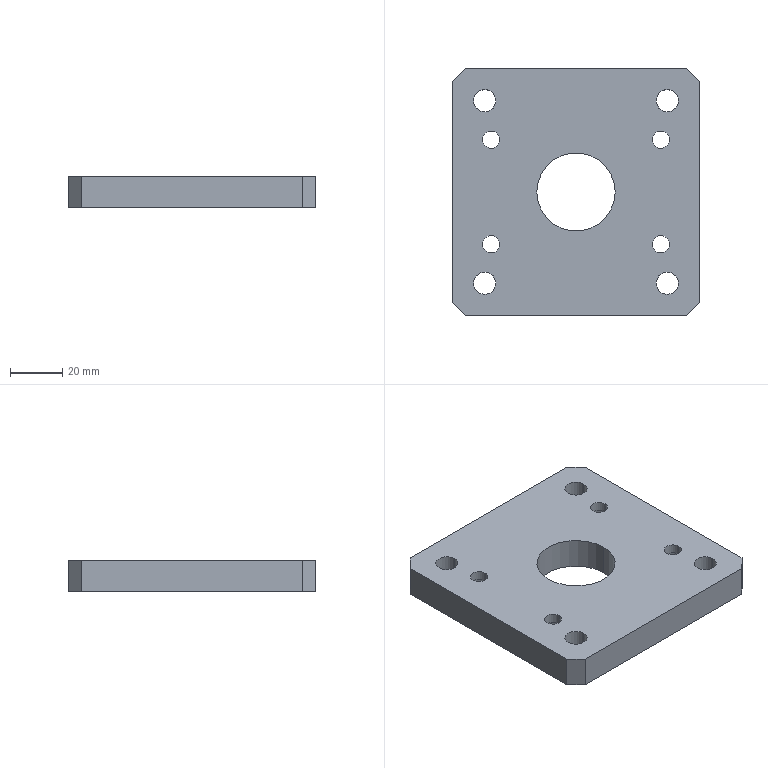Part | SolidWorks | features 3DProfileFeature 3, HoleWzd 3, Chamfer 1, Extrusion 1, ICE 1 | 1 solid | 40 faces | box 95 x 95 x 12 mm | volume 92833 mm3 | cylinder 26 | plane 14 | commonest cylinder face diameters 6.6 x8 8.5 x8 11 x8 30 x2
STEP:
#1=CARTESIAN_POINT('',(87.554,35.,12.));
#2=VERTEX_POINT('',#1);
#3=CARTESIAN_POINT('',(79.054,35.,12.));
#4=VERTEX_POINT('',#3);
#5=CARTESIAN_POINT('',(83.304,35.,12.));
#6=DIRECTION('',(0.,0.,-1.));
#7=DIRECTION('',(-1.,0.,0.));
#8=AXIS2_PLACEMENT_3D('',#5,#6,#7);
#9=CIRCLE('',#8,4.25);
#10=EDGE_CURVE('',#2,#4,#9,.T.);
#11=ORIENTED_EDGE('',*,*,#10,.F.);
#12=CARTESIAN_POINT('',(87.554,35.,0.));
#13=VERTEX_POINT('',#12);
#14=CARTESIAN_POINT('',(87.554,35.,0.));
#15=DIRECTION('',(0.,0.,-1.));
#16=VECTOR('',#15,1000.);
#17=LINE('',#14,#16);
#18=EDGE_CURVE('',#2,#13,#17,.T.);
#19=ORIENTED_EDGE('',*,*,#18,.T.);
#20=CARTESIAN_POINT('',(79.054,35.,0.));
#21=VERTEX_POINT('',#20);
#22=CARTESIAN_POINT('',(83.304,35.,0.));
#23=DIRECTION('',(0.,0.,-1.));
#24=DIRECTION('',(-1.,0.,0.));
#25=AXIS2_PLACEMENT_3D('',#22,#23,#24);
#26=CIRCLE('',#25,4.25);
#27=EDGE_CURVE('',#13,#21,#26,.T.);
#28=ORIENTED_EDGE('',*,*,#27,.T.);
#29=CARTESIAN_POINT('',(79.054,35.,0.));
#30=DIRECTION('',(0.,0.,-1.));
#31=VECTOR('',#30,1000.);
#32=LINE('',#29,#31);
#33=EDGE_CURVE('',#4,#21,#32,.T.);
#34=ORIENTED_EDGE('',*,*,#33,.F.);
#35=EDGE_LOOP('',(#11,#19,#28,#34));
#36=FACE_OUTER_BOUND('',#35,.T.);
#37=CARTESIAN_POINT('',(83.304,35.,0.));
#38=DIRECTION('',(0.,0.,-1.));
#39=DIRECTION('',(-1.,0.,0.));
#40=AXIS2_PLACEMENT_3D('',#37,#38,#39);
#41=CYLINDRICAL_SURFACE('',#40,4.25);
#42=ADVANCED_FACE('',(#36),#41,.F.);
#43=CARTESIAN_POINT('',(17.554,35.,12.));
#44=VERTEX_POINT('',#43);
#45=CARTESIAN_POINT('',(9.054,35.,12.));
#46=VERTEX_POINT('',#45);
#47=CARTESIAN_POINT('',(13.304,35.,12.));
#48=DIRECTION('',(0.,0.,-1.));
#49=DIRECTION('',(-1.,0.,0.));
#50=AXIS2_PLACEMENT_3D('',#47,#48,#49);
#51=CIRCLE('',#50,4.25);
#52=EDGE_CURVE('',#44,#46,#51,.T.);
#53=ORIENTED_EDGE('',*,*,#52,.F.);
#54=CARTESIAN_POINT('',(17.554,35.,0.));
#55=VERTEX_POINT('',#54);
#56=CARTESIAN_POINT('',(17.554,35.,0.));
#57=DIRECTION('',(0.,0.,-1.));
#58=VECTOR('',#57,1000.);
#59=LINE('',#56,#58);
#60=EDGE_CURVE('',#44,#55,#59,.T.);
#61=ORIENTED_EDGE('',*,*,#60,.T.);
#62=CARTESIAN_POINT('',(9.054,35.,0.));
#63=VERTEX_POINT('',#62);
#64=CARTESIAN_POINT('',(13.304,35.,0.));
#65=DIRECTION('',(0.,0.,-1.));
#66=DIRECTION('',(-1.,0.,0.));
#67=AXIS2_PLACEMENT_3D('',#64,#65,#66);
#68=CIRCLE('',#67,4.25);
#69=EDGE_CURVE('',#55,#63,#68,.T.);
#70=ORIENTED_EDGE('',*,*,#69,.T.);
#71=CARTESIAN_POINT('',(9.054,35.,0.));
#72=DIRECTION('',(0.,0.,-1.));
#73=VECTOR('',#72,1000.);
#74=LINE('',#71,#73);
#75=EDGE_CURVE('',#46,#63,#74,.T.);
#76=ORIENTED_EDGE('',*,*,#75,.F.);
#77=EDGE_LOOP('',(#53,#61,#70,#76));
#78=FACE_OUTER_BOUND('',#77,.T.);
#79=CARTESIAN_POINT('',(13.304,35.,0.));
#80=DIRECTION('',(0.,0.,-1.));
#81=DIRECTION('',(-1.,0.,0.));
#82=AXIS2_PLACEMENT_3D('',#79,#80,#81);
#83=CYLINDRICAL_SURFACE('',#82,4.25);
#84=ADVANCED_FACE('',(#78),#83,.F.);
#85=CARTESIAN_POINT('',(17.554,-35.,12.));
#86=VERTEX_POINT('',#85);
#87=CARTESIAN_POINT('',(9.054,-35.,12.));
#88=VERTEX_POINT('',#87);
#89=CARTESIAN_POINT('',(13.304,-35.,12.));
#90=DIRECTION('',(0.,0.,-1.));
#91=DIRECTION('',(-1.,0.,0.));
#92=AXIS2_PLACEMENT_3D('',#89,#90,#91);
#93=CIRCLE('',#92,4.25);
#94=EDGE_CURVE('',#86,#88,#93,.T.);
#95=ORIENTED_EDGE('',*,*,#94,.F.);
#96=CARTESIAN_POINT('',(17.554,-35.,0.));
#97=VERTEX_POINT('',#96);
#98=CARTESIAN_POINT('',(17.554,-35.,0.));
#99=DIRECTION('',(0.,0.,-1.));
#100=VECTOR('',#99,1000.);
#101=LINE('',#98,#100);
#102=EDGE_CURVE('',#86,#97,#101,.T.);
#103=ORIENTED_EDGE('',*,*,#102,.T.);
#104=CARTESIAN_POINT('',(9.054,-35.,0.));
#105=VERTEX_POINT('',#104);
#106=CARTESIAN_POINT('',(13.304,-35.,0.));
#107=DIRECTION('',(0.,0.,-1.));
#108=DIRECTION('',(-1.,0.,0.));
#109=AXIS2_PLACEMENT_3D('',#106,#107,#108);
#110=CIRCLE('',#109,4.25);
#111=EDGE_CURVE('',#97,#105,#110,.T.);
#112=ORIENTED_EDGE('',*,*,#111,.T.);
#113=CARTESIAN_POINT('',(9.054,-35.,0.));
#114=DIRECTION('',(0.,0.,-1.));
#115=VECTOR('',#114,1000.);
#116=LINE('',#113,#115);
#117=EDGE_CURVE('',#88,#105,#116,.T.);
#118=ORIENTED_EDGE('',*,*,#117,.F.);
#119=EDGE_LOOP('',(#95,#103,#112,#118));
#120=FACE_OUTER_BOUND('',#119,.T.);
#121=CARTESIAN_POINT('',(13.304,-35.,0.));
#122=DIRECTION('',(0.,0.,-1.));
#123=DIRECTION('',(-1.,0.,0.));
#124=AXIS2_PLACEMENT_3D('',#121,#122,#123);
#125=CYLINDRICAL_SURFACE('',#124,4.25);
#126=ADVANCED_FACE('',(#120),#125,.F.);
#127=CARTESIAN_POINT('',(87.554,-35.,12.));
#128=VERTEX_POINT('',#127);
#129=CARTESIAN_POINT('',(79.054,-35.,12.));
#130=VERTEX_POINT('',#129);
#131=CARTESIAN_POINT('',(83.304,-35.,12.));
#132=DIRECTION('',(0.,0.,-1.));
#133=DIRECTION('',(-1.,0.,0.));
#134=AXIS2_PLACEMENT_3D('',#131,#132,#133);
#135=CIRCLE('',#134,4.25);
#136=EDGE_CURVE('',#128,#130,#135,.T.);
#137=ORIENTED_EDGE('',*,*,#136,.F.);
#138=CARTESIAN_POINT('',(87.554,-35.,0.));
#139=VERTEX_POINT('',#138);
#140=CARTESIAN_POINT('',(87.554,-35.,0.));
#141=DIRECTION('',(0.,0.,-1.));
#142=VECTOR('',#141,1000.);
#143=LINE('',#140,#142);
#144=EDGE_CURVE('',#128,#139,#143,.T.);
#145=ORIENTED_EDGE('',*,*,#144,.T.);
#146=CARTESIAN_POINT('',(79.054,-35.,0.));
#147=VERTEX_POINT('',#146);
#148=CARTESIAN_POINT('',(83.304,-35.,0.));
#149=DIRECTION('',(0.,0.,-1.));
#150=DIRECTION('',(-1.,0.,0.));
#151=AXIS2_PLACEMENT_3D('',#148,#149,#150);
#152=CIRCLE('',#151,4.25);
#153=EDGE_CURVE('',#139,#147,#152,.T.);
#154=ORIENTED_EDGE('',*,*,#153,.T.);
#155=CARTESIAN_POINT('',(79.054,-35.,0.));
#156=DIRECTION('',(0.,0.,-1.));
#157=VECTOR('',#156,1000.);
#158=LINE('',#155,#157);
#159=EDGE_CURVE('',#130,#147,#158,.T.);
#160=ORIENTED_EDGE('',*,*,#159,.F.);
#161=EDGE_LOOP('',(#137,#145,#154,#160));
#162=FACE_OUTER_BOUND('',#161,.T.);
#163=CARTESIAN_POINT('',(83.304,-35.,0.));
#164=DIRECTION('',(0.,0.,-1.));
#165=DIRECTION('',(-1.,0.,0.));
#166=AXIS2_PLACEMENT_3D('',#163,#164,#165);
#167=CYLINDRICAL_SURFACE('',#166,4.25);
#168=ADVANCED_FACE('',(#162),#167,.F.);
#169=CARTESIAN_POINT('',(86.304,20.,8.3));
#170=VERTEX_POINT('',#169);
#171=CARTESIAN_POINT('',(75.304,20.,8.3));
#172=VERTEX_POINT('',#171);
#173=CARTESIAN_POINT('',(80.804,20.,8.3));
#174=DIRECTION('',(0.,0.,-1.));
#175=DIRECTION('',(-1.,0.,0.));
#176=AXIS2_PLACEMENT_3D('',#173,#174,#175);
#177=CIRCLE('',#176,5.5);
#178=EDGE_CURVE('',#170,#172,#177,.T.);
#179=ORIENTED_EDGE('',*,*,#178,.F.);
#180=CARTESIAN_POINT('',(86.304,20.,0.));
#181=VERTEX_POINT('',#180);
#182=CARTESIAN_POINT('',(86.304,20.,0.));
#183=DIRECTION('',(0.,0.,-1.));
#184=VECTOR('',#183,1000.);
#185=LINE('',#182,#184);
#186=EDGE_CURVE('',#170,#181,#185,.T.);
#187=ORIENTED_EDGE('',*,*,#186,.T.);
#188=CARTESIAN_POINT('',(75.304,20.,0.));
#189=VERTEX_POINT('',#188);
#190=CARTESIAN_POINT('',(80.804,20.,0.));
#191=DIRECTION('',(0.,0.,-1.));
#192=DIRECTION('',(-1.,0.,0.));
#193=AXIS2_PLACEMENT_3D('',#190,#191,#192);
#194=CIRCLE('',#193,5.5);
#195=EDGE_CURVE('',#181,#189,#194,.T.);
#196=ORIENTED_EDGE('',*,*,#195,.T.);
#197=CARTESIAN_POINT('',(75.304,20.,0.));
#198=DIRECTION('',(0.,0.,-1.));
#199=VECTOR('',#198,1000.);
#200=LINE('',#197,#199);
#201=EDGE_CURVE('',#172,#189,#200,.T.);
#202=ORIENTED_EDGE('',*,*,#201,.F.);
#203=EDGE_LOOP('',(#179,#187,#196,#202));
#204=FACE_OUTER_BOUND('',#203,.T.);
#205=CARTESIAN_POINT('',(80.804,20.,0.));
#206=DIRECTION('',(0.,0.,-1.));
#207=DIRECTION('',(-1.,0.,0.));
#208=AXIS2_PLACEMENT_3D('',#205,#206,#207);
#209=CYLINDRICAL_SURFACE('',#208,5.5);
#210=ADVANCED_FACE('',(#204),#209,.F.);
#211=CARTESIAN_POINT('',(84.104,20.,12.));
#212=VERTEX_POINT('',#211);
#213=CARTESIAN_POINT('',(77.504,20.,12.));
#214=VERTEX_POINT('',#213);
#215=CARTESIAN_POINT('',(80.804,20.,12.));
#216=DIRECTION('',(0.,0.,-1.));
#217=DIRECTION('',(-1.,0.,0.));
#218=AXIS2_PLACEMENT_3D('',#215,#216,#217);
#219=CIRCLE('',#218,3.3);
#220=EDGE_CURVE('',#212,#214,#219,.T.);
#221=ORIENTED_EDGE('',*,*,#220,.F.);
#222=CARTESIAN_POINT('',(84.104,20.,8.3));
#223=VERTEX_POINT('',#222);
#224=CARTESIAN_POINT('',(84.104,20.,0.));
#225=DIRECTION('',(0.,0.,-1.));
#226=VECTOR('',#225,1000.);
#227=LINE('',#224,#226);
#228=EDGE_CURVE('',#212,#223,#227,.T.);
#229=ORIENTED_EDGE('',*,*,#228,.T.);
#230=CARTESIAN_POINT('',(77.504,20.,8.3));
#231=VERTEX_POINT('',#230);
#232=CARTESIAN_POINT('',(80.804,20.,8.3));
#233=DIRECTION('',(0.,0.,-1.));
#234=DIRECTION('',(-1.,0.,0.));
#235=AXIS2_PLACEMENT_3D('',#232,#233,#234);
#236=CIRCLE('',#235,3.3);
#237=EDGE_CURVE('',#223,#231,#236,.T.);
#238=ORIENTED_EDGE('',*,*,#237,.T.);
#239=CARTESIAN_POINT('',(77.504,20.,0.));
#240=DIRECTION('',(0.,0.,-1.));
#241=VECTOR('',#240,1000.);
#242=LINE('',#239,#241);
#243=EDGE_CURVE('',#214,#231,#242,.T.);
#244=ORIENTED_EDGE('',*,*,#243,.F.);
#245=EDGE_LOOP('',(#221,#229,#238,#244));
#246=FACE_OUTER_BOUND('',#245,.T.);
#247=CARTESIAN_POINT('',(80.804,20.,0.));
#248=DIRECTION('',(0.,0.,-1.));
#249=DIRECTION('',(-1.,0.,0.));
#250=AXIS2_PLACEMENT_3D('',#247,#248,#249);
#251=CYLINDRICAL_SURFACE('',#250,3.3);
#252=ADVANCED_FACE('',(#246),#251,.F.);
#253=CARTESIAN_POINT('',(21.304,20.,8.3));
#254=VERTEX_POINT('',#253);
#255=CARTESIAN_POINT('',(10.304,20.,8.3));
#256=VERTEX_POINT('',#255);
#257=CARTESIAN_POINT('',(15.804,20.,8.3));
#258=DIRECTION('',(0.,0.,-1.));
#259=DIRECTION('',(-1.,0.,0.));
#260=AXIS2_PLACEMENT_3D('',#257,#258,#259);
#261=CIRCLE('',#260,5.5);
#262=EDGE_CURVE('',#254,#256,#261,.T.);
#263=ORIENTED_EDGE('',*,*,#262,.F.);
#264=CARTESIAN_POINT('',(21.304,20.,0.));
#265=VERTEX_POINT('',#264);
#266=CARTESIAN_POINT('',(21.304,20.,0.));
#267=DIRECTION('',(0.,0.,-1.));
#268=VECTOR('',#267,1000.);
#269=LINE('',#266,#268);
#270=EDGE_CURVE('',#254,#265,#269,.T.);
#271=ORIENTED_EDGE('',*,*,#270,.T.);
#272=CARTESIAN_POINT('',(10.304,20.,0.));
#273=VERTEX_POINT('',#272);
#274=CARTESIAN_POINT('',(15.804,20.,0.));
#275=DIRECTION('',(0.,0.,-1.));
#276=DIRECTION('',(-1.,0.,0.));
#277=AXIS2_PLACEMENT_3D('',#274,#275,#276);
#278=CIRCLE('',#277,5.5);
#279=EDGE_CURVE('',#265,#273,#278,.T.);
#280=ORIENTED_EDGE('',*,*,#279,.T.);
#281=CARTESIAN_POINT('',(10.304,20.,0.));
#282=DIRECTION('',(0.,0.,-1.));
#283=VECTOR('',#282,1000.);
#284=LINE('',#281,#283);
#285=EDGE_CURVE('',#256,#273,#284,.T.);
#286=ORIENTED_EDGE('',*,*,#285,.F.);
#287=EDGE_LOOP('',(#263,#271,#280,#286));
#288=FACE_OUTER_BOUND('',#287,.T.);
#289=CARTESIAN_POINT('',(15.804,20.,0.));
#290=DIRECTION('',(0.,0.,-1.));
#291=DIRECTION('',(-1.,0.,0.));
#292=AXIS2_PLACEMENT_3D('',#289,#290,#291);
#293=CYLINDRICAL_SURFACE('',#292,5.5);
#294=ADVANCED_FACE('',(#288),#293,.F.);
#295=CARTESIAN_POINT('',(19.104,20.,12.));
#296=VERTEX_POINT('',#295);
#297=CARTESIAN_POINT('',(12.504,20.,12.));
#298=VERTEX_POINT('',#297);
#299=CARTESIAN_POINT('',(15.804,20.,12.));
#300=DIRECTION('',(0.,0.,-1.));
#301=DIRECTION('',(-1.,0.,0.));
#302=AXIS2_PLACEMENT_3D('',#299,#300,#301);
#303=CIRCLE('',#302,3.3);
#304=EDGE_CURVE('',#296,#298,#303,.T.);
#305=ORIENTED_EDGE('',*,*,#304,.F.);
#306=CARTESIAN_POINT('',(19.104,20.,8.3));
#307=VERTEX_POINT('',#306);
#308=CARTESIAN_POINT('',(19.104,20.,0.));
#309=DIRECTION('',(0.,0.,-1.));
#310=VECTOR('',#309,1000.);
#311=LINE('',#308,#310);
#312=EDGE_CURVE('',#296,#307,#311,.T.);
#313=ORIENTED_EDGE('',*,*,#312,.T.);
#314=CARTESIAN_POINT('',(12.504,20.,8.3));
#315=VERTEX_POINT('',#314);
#316=CARTESIAN_POINT('',(15.804,20.,8.3));
#317=DIRECTION('',(0.,0.,-1.));
#318=DIRECTION('',(-1.,0.,0.));
#319=AXIS2_PLACEMENT_3D('',#316,#317,#318);
#320=CIRCLE('',#319,3.3);
#321=EDGE_CURVE('',#307,#315,#320,.T.);
#322=ORIENTED_EDGE('',*,*,#321,.T.);
#323=CARTESIAN_POINT('',(12.504,20.,0.));
#324=DIRECTION('',(0.,0.,-1.));
#325=VECTOR('',#324,1000.);
#326=LINE('',#323,#325);
#327=EDGE_CURVE('',#298,#315,#326,.T.);
#328=ORIENTED_EDGE('',*,*,#327,.F.);
#329=EDGE_LOOP('',(#305,#313,#322,#328));
#330=FACE_OUTER_BOUND('',#329,.T.);
#331=CARTESIAN_POINT('',(15.804,20.,0.));
#332=DIRECTION('',(0.,0.,-1.));
#333=DIRECTION('',(-1.,0.,0.));
#334=AXIS2_PLACEMENT_3D('',#331,#332,#333);
#335=CYLINDRICAL_SURFACE('',#334,3.3);
#336=ADVANCED_FACE('',(#330),#335,.F.);
#337=CARTESIAN_POINT('',(21.304,-20.,8.3));
#338=VERTEX_POINT('',#337);
#339=CARTESIAN_POINT('',(10.304,-20.,8.3));
#340=VERTEX_POINT('',#339);
#341=CARTESIAN_POINT('',(15.804,-20.,8.3));
#342=DIRECTION('',(0.,0.,-1.));
#343=DIRECTION('',(-1.,0.,0.));
#344=AXIS2_PLACEMENT_3D('',#341,#342,#343);
#345=CIRCLE('',#344,5.5);
#346=EDGE_CURVE('',#338,#340,#345,.T.);
#347=ORIENTED_EDGE('',*,*,#346,.F.);
#348=CARTESIAN_POINT('',(21.304,-20.,0.));
#349=VERTEX_POINT('',#348);
#350=CARTESIAN_POINT('',(21.304,-20.,0.));
#351=DIRECTION('',(0.,0.,-1.));
#352=VECTOR('',#351,1000.);
#353=LINE('',#350,#352);
#354=EDGE_CURVE('',#338,#349,#353,.T.);
#355=ORIENTED_EDGE('',*,*,#354,.T.);
#356=CARTESIAN_POINT('',(10.304,-20.,0.));
#357=VERTEX_POINT('',#356);
#358=CARTESIAN_POINT('',(15.804,-20.,0.));
#359=DIRECTION('',(0.,0.,-1.));
#360=DIRECTION('',(-1.,0.,0.));
#361=AXIS2_PLACEMENT_3D('',#358,#359,#360);
#362=CIRCLE('',#361,5.5);
#363=EDGE_CURVE('',#349,#357,#362,.T.);
#364=ORIENTED_EDGE('',*,*,#363,.T.);
#365=CARTESIAN_POINT('',(10.304,-20.,0.));
#366=DIRECTION('',(0.,0.,-1.));
#367=VECTOR('',#366,1000.);
#368=LINE('',#365,#367);
#369=EDGE_CURVE('',#340,#357,#368,.T.);
#370=ORIENTED_EDGE('',*,*,#369,.F.);
#371=EDGE_LOOP('',(#347,#355,#364,#370));
#372=FACE_OUTER_BOUND('',#371,.T.);
#373=CARTESIAN_POINT('',(15.804,-20.,0.));
#374=DIRECTION('',(0.,0.,-1.));
#375=DIRECTION('',(-1.,0.,0.));
#376=AXIS2_PLACEMENT_3D('',#373,#374,#375);
#377=CYLINDRICAL_SURFACE('',#376,5.5);
#378=ADVANCED_FACE('',(#372),#377,.F.);
#379=CARTESIAN_POINT('',(19.104,-20.,12.));
#380=VERTEX_POINT('',#379);
#381=CARTESIAN_POINT('',(12.504,-20.,12.));
#382=VERTEX_POINT('',#381);
#383=CARTESIAN_POINT('',(15.804,-20.,12.));
#384=DIRECTION('',(0.,0.,-1.));
#385=DIRECTION('',(-1.,0.,0.));
#386=AXIS2_PLACEMENT_3D('',#383,#384,#385);
#387=CIRCLE('',#386,3.3);
#388=EDGE_CURVE('',#380,#382,#387,.T.);
#389=ORIENTED_EDGE('',*,*,#388,.F.);
#390=CARTESIAN_POINT('',(19.104,-20.,8.3));
#391=VERTEX_POINT('',#390);
#392=CARTESIAN_POINT('',(19.104,-20.,0.));
#393=DIRECTION('',(0.,0.,-1.));
#394=VECTOR('',#393,1000.);
#395=LINE('',#392,#394);
#396=EDGE_CURVE('',#380,#391,#395,.T.);
#397=ORIENTED_EDGE('',*,*,#396,.T.);
#398=CARTESIAN_POINT('',(12.504,-20.,8.3));
#399=VERTEX_POINT('',#398);
#400=CARTESIAN_POINT('',(15.804,-20.,8.3));
#401=DIRECTION('',(0.,0.,-1.));
#402=DIRECTION('',(-1.,0.,0.));
#403=AXIS2_PLACEMENT_3D('',#400,#401,#402);
#404=CIRCLE('',#403,3.3);
#405=EDGE_CURVE('',#391,#399,#404,.T.);
#406=ORIENTED_EDGE('',*,*,#405,.T.);
#407=CARTESIAN_POINT('',(12.504,-20.,0.));
#408=DIRECTION('',(0.,0.,-1.));
#409=VECTOR('',#408,1000.);
#410=LINE('',#407,#409);
#411=EDGE_CURVE('',#382,#399,#410,.T.);
#412=ORIENTED_EDGE('',*,*,#411,.F.);
#413=EDGE_LOOP('',(#389,#397,#406,#412));
#414=FACE_OUTER_BOUND('',#413,.T.);
#415=CARTESIAN_POINT('',(15.804,-20.,0.));
#416=DIRECTION('',(0.,0.,-1.));
#417=DIRECTION('',(-1.,0.,0.));
#418=AXIS2_PLACEMENT_3D('',#415,#416,#417);
#419=CYLINDRICAL_SURFACE('',#418,3.3);
#420=ADVANCED_FACE('',(#414),#419,.F.);
#421=CARTESIAN_POINT('',(86.304,-20.,8.3));
#422=VERTEX_POINT('',#421);
#423=CARTESIAN_POINT('',(75.304,-20.,8.3));
#424=VERTEX_POINT('',#423);
#425=CARTESIAN_POINT('',(80.804,-20.,8.3));
#426=DIRECTION('',(0.,0.,-1.));
#427=DIRECTION('',(-1.,0.,0.));
#428=AXIS2_PLACEMENT_3D('',#425,#426,#427);
#429=CIRCLE('',#428,5.5);
#430=EDGE_CURVE('',#422,#424,#429,.T.);
#431=ORIENTED_EDGE('',*,*,#430,.F.);
#432=CARTESIAN_POINT('',(86.304,-20.,0.));
#433=VERTEX_POINT('',#432);
#434=CARTESIAN_POINT('',(86.304,-20.,0.));
#435=DIRECTION('',(0.,0.,-1.));
#436=VECTOR('',#435,1000.);
#437=LINE('',#434,#436);
#438=EDGE_CURVE('',#422,#433,#437,.T.);
#439=ORIENTED_EDGE('',*,*,#438,.T.);
#440=CARTESIAN_POINT('',(75.304,-20.,0.));
#441=VERTEX_POINT('',#440);
#442=CARTESIAN_POINT('',(80.804,-20.,0.));
#443=DIRECTION('',(0.,0.,-1.));
#444=DIRECTION('',(-1.,0.,0.));
#445=AXIS2_PLACEMENT_3D('',#442,#443,#444);
#446=CIRCLE('',#445,5.5);
#447=EDGE_CURVE('',#433,#441,#446,.T.);
#448=ORIENTED_EDGE('',*,*,#447,.T.);
#449=CARTESIAN_POINT('',(75.304,-20.,0.));
#450=DIRECTION('',(0.,0.,-1.));
#451=VECTOR('',#450,1000.);
#452=LINE('',#449,#451);
#453=EDGE_CURVE('',#424,#441,#452,.T.);
#454=ORIENTED_EDGE('',*,*,#453,.F.);
#455=EDGE_LOOP('',(#431,#439,#448,#454));
#456=FACE_OUTER_BOUND('',#455,.T.);
#457=CARTESIAN_POINT('',(80.804,-20.,0.));
#458=DIRECTION('',(0.,0.,-1.));
#459=DIRECTION('',(-1.,0.,0.));
#460=AXIS2_PLACEMENT_3D('',#457,#458,#459);
#461=CYLINDRICAL_SURFACE('',#460,5.5);
#462=ADVANCED_FACE('',(#456),#461,.F.);
#463=CARTESIAN_POINT('',(84.104,-20.,12.));
#464=VERTEX_POINT('',#463);
#465=CARTESIAN_POINT('',(77.504,-20.,12.));
#466=VERTEX_POINT('',#465);
#467=CARTESIAN_POINT('',(80.804,-20.,12.));
#468=DIRECTION('',(0.,0.,-1.));
#469=DIRECTION('',(-1.,0.,0.));
#470=AXIS2_PLACEMENT_3D('',#467,#468,#469);
#471=CIRCLE('',#470,3.3);
#472=EDGE_CURVE('',#464,#466,#471,.T.);
#473=ORIENTED_EDGE('',*,*,#472,.F.);
#474=CARTESIAN_POINT('',(84.104,-20.,8.3));
#475=VERTEX_POINT('',#474);
#476=CARTESIAN_POINT('',(84.104,-20.,0.));
#477=DIRECTION('',(0.,0.,-1.));
#478=VECTOR('',#477,1000.);
#479=LINE('',#476,#478);
#480=EDGE_CURVE('',#464,#475,#479,.T.);
#481=ORIENTED_EDGE('',*,*,#480,.T.);
#482=CARTESIAN_POINT('',(77.504,-20.,8.3));
#483=VERTEX_POINT('',#482);
#484=CARTESIAN_POINT('',(80.804,-20.,8.3));
#485=DIRECTION('',(0.,0.,-1.));
#486=DIRECTION('',(-1.,0.,0.));
#487=AXIS2_PLACEMENT_3D('',#484,#485,#486);
#488=CIRCLE('',#487,3.3);
#489=EDGE_CURVE('',#475,#483,#488,.T.);
#490=ORIENTED_EDGE('',*,*,#489,.T.);
#491=CARTESIAN_POINT('',(77.504,-20.,0.));
#492=DIRECTION('',(0.,0.,-1.));
#493=VECTOR('',#492,1000.);
#494=LINE('',#491,#493);
#495=EDGE_CURVE('',#466,#483,#494,.T.);
#496=ORIENTED_EDGE('',*,*,#495,.F.);
#497=EDGE_LOOP('',(#473,#481,#490,#496));
#498=FACE_OUTER_BOUND('',#497,.T.);
#499=CARTESIAN_POINT('',(80.804,-20.,0.));
#500=DIRECTION('',(0.,0.,-1.));
#501=DIRECTION('',(-1.,0.,0.));
#502=AXIS2_PLACEMENT_3D('',#499,#500,#501);
#503=CYLINDRICAL_SURFACE('',#502,3.3);
#504=ADVANCED_FACE('',(#498),#503,.F.);
#505=CARTESIAN_POINT('',(33.304,0.,0.));
#506=VERTEX_POINT('',#505);
#507=CARTESIAN_POINT('',(63.304,0.,0.));
#508=VERTEX_POINT('',#507);
#509=CARTESIAN_POINT('',(48.304,0.,0.));
#510=DIRECTION('',(0.,0.,1.));
#511=DIRECTION('',(1.,0.,0.));
#512=AXIS2_PLACEMENT_3D('',#509,#510,#511);
#513=CIRCLE('',#512,15.);
#514=EDGE_CURVE('',#506,#508,#513,.T.);
#515=ORIENTED_EDGE('',*,*,#514,.F.);
#516=CARTESIAN_POINT('',(33.304,0.,12.));
#517=VERTEX_POINT('',#516);
#518=CARTESIAN_POINT('',(33.304,0.,0.));
#519=DIRECTION('',(0.,0.,1.));
#520=VECTOR('',#519,1000.);
#521=LINE('',#518,#520);
#522=EDGE_CURVE('',#506,#517,#521,.T.);
#523=ORIENTED_EDGE('',*,*,#522,.T.);
#524=CARTESIAN_POINT('',(63.304,0.,12.));
#525=VERTEX_POINT('',#524);
#526=CARTESIAN_POINT('',(48.304,0.,12.));
#527=DIRECTION('',(0.,0.,1.));
#528=DIRECTION('',(1.,0.,0.));
#529=AXIS2_PLACEMENT_3D('',#526,#527,#528);
#530=CIRCLE('',#529,15.);
#531=EDGE_CURVE('',#517,#525,#530,.T.);
#532=ORIENTED_EDGE('',*,*,#531,.T.);
#533=CARTESIAN_POINT('',(63.304,0.,0.));
#534=DIRECTION('',(0.,0.,1.));
#535=VECTOR('',#534,1000.);
#536=LINE('',#533,#535);
#537=EDGE_CURVE('',#508,#525,#536,.T.);
#538=ORIENTED_EDGE('',*,*,#537,.F.);
#539=EDGE_LOOP('',(#515,#523,#532,#538));
#540=FACE_OUTER_BOUND('',#539,.T.);
#541=CARTESIAN_POINT('',(48.304,0.,0.));
#542=DIRECTION('',(0.,0.,1.));
#543=DIRECTION('',(1.,0.,0.));
#544=AXIS2_PLACEMENT_3D('',#541,#542,#543);
#545=CYLINDRICAL_SURFACE('',#544,15.);
#546=ADVANCED_FACE('',(#540),#545,.F.);
#547=CARTESIAN_POINT('',(0.8045,42.5,12.));
#548=VERTEX_POINT('',#547);
#549=CARTESIAN_POINT('',(0.8045,-42.5,12.));
#550=VERTEX_POINT('',#549);
#551=CARTESIAN_POINT('',(0.8045,-47.5,12.));
#552=DIRECTION('',(0.,-1.,0.));
#553=VECTOR('',#552,1000.);
#554=LINE('',#551,#553);
#555=EDGE_CURVE('',#548,#550,#554,.T.);
#556=ORIENTED_EDGE('',*,*,#555,.F.);
#557=CARTESIAN_POINT('',(0.8045,42.5,0.));
#558=VERTEX_POINT('',#557);
#559=CARTESIAN_POINT('',(0.8045,42.5,12.));
#560=DIRECTION('',(0.,0.,-1.));
#561=VECTOR('',#560,1000.);
#562=LINE('',#559,#561);
#563=EDGE_CURVE('',#548,#558,#562,.T.);
#564=ORIENTED_EDGE('',*,*,#563,.T.);
#565=CARTESIAN_POINT('',(0.8045,-42.5,0.));
#566=VERTEX_POINT('',#565);
#567=CARTESIAN_POINT('',(0.8045,-47.5,0.));
#568=DIRECTION('',(0.,-1.,0.));
#569=VECTOR('',#568,1000.);
#570=LINE('',#567,#569);
#571=EDGE_CURVE('',#558,#566,#570,.T.);
#572=ORIENTED_EDGE('',*,*,#571,.T.);
#573=CARTESIAN_POINT('',(0.8045,-42.5,12.));
#574=DIRECTION('',(0.,0.,1.));
#575=VECTOR('',#574,1000.);
#576=LINE('',#573,#575);
#577=EDGE_CURVE('',#566,#550,#576,.T.);
#578=ORIENTED_EDGE('',*,*,#577,.T.);
#579=EDGE_LOOP('',(#556,#564,#572,#578));
#580=FACE_OUTER_BOUND('',#579,.T.);
#581=CARTESIAN_POINT('',(0.8045,-47.5,12.));
#582=DIRECTION('',(1.,0.,0.));
#583=DIRECTION('',(0.,0.,-1.));
#584=AXIS2_PLACEMENT_3D('',#581,#582,#583);
#585=PLANE('',#584);
#586=ADVANCED_FACE('',(#580),#585,.F.);
#587=CARTESIAN_POINT('',(5.804,-47.5,0.));
#588=VERTEX_POINT('',#587);
#589=CARTESIAN_POINT('',(90.804,-47.5,0.));
#590=VERTEX_POINT('',#589);
#591=CARTESIAN_POINT('',(0.8045,-47.5,0.));
#592=DIRECTION('',(1.,0.,0.));
#593=VECTOR('',#592,1000.);
#594=LINE('',#591,#593);
#595=EDGE_CURVE('',#588,#590,#594,.T.);
#596=ORIENTED_EDGE('',*,*,#595,.T.);
#597=CARTESIAN_POINT('',(90.804,-47.5,12.));
#598=VERTEX_POINT('',#597);
#599=CARTESIAN_POINT('',(90.804,-47.5,12.));
#600=DIRECTION('',(0.,0.,1.));
#601=VECTOR('',#600,1000.);
#602=LINE('',#599,#601);
#603=EDGE_CURVE('',#590,#598,#602,.T.);
#604=ORIENTED_EDGE('',*,*,#603,.T.);
#605=CARTESIAN_POINT('',(5.804,-47.5,12.));
#606=VERTEX_POINT('',#605);
#607=CARTESIAN_POINT('',(0.8045,-47.5,12.));
#608=DIRECTION('',(1.,0.,0.));
#609=VECTOR('',#608,1000.);
#610=LINE('',#607,#609);
#611=EDGE_CURVE('',#606,#598,#610,.T.);
#612=ORIENTED_EDGE('',*,*,#611,.F.);
#613=CARTESIAN_POINT('',(5.804,-47.5,12.));
#614=DIRECTION('',(0.,0.,-1.));
#615=VECTOR('',#614,1000.);
#616=LINE('',#613,#615);
#617=EDGE_CURVE('',#606,#588,#616,.T.);
#618=ORIENTED_EDGE('',*,*,#617,.T.);
#619=EDGE_LOOP('',(#596,#604,#612,#618));
#620=FACE_OUTER_BOUND('',#619,.T.);
#621=CARTESIAN_POINT('',(0.8045,-47.5,12.));
#622=DIRECTION('',(0.,1.,0.));
#623=DIRECTION('',(0.,0.,1.));
#624=AXIS2_PLACEMENT_3D('',#621,#622,#623);
#625=PLANE('',#624);
#626=ADVANCED_FACE('',(#620),#625,.F.);
#627=CARTESIAN_POINT('',(95.804,-42.5,0.));
#628=VERTEX_POINT('',#627);
#629=CARTESIAN_POINT('',(95.804,42.5,0.));
#630=VERTEX_POINT('',#629);
#631=CARTESIAN_POINT('',(95.804,-47.5,0.));
#632=DIRECTION('',(0.,1.,0.));
#633=VECTOR('',#632,1000.);
#634=LINE('',#631,#633);
#635=EDGE_CURVE('',#628,#630,#634,.T.);
#636=ORIENTED_EDGE('',*,*,#635,.T.);
#637=CARTESIAN_POINT('',(95.804,42.5,12.));
#638=VERTEX_POINT('',#637);
#639=CARTESIAN_POINT('',(95.804,42.5,12.));
#640=DIRECTION('',(0.,0.,1.));
#641=VECTOR('',#640,1000.);
#642=LINE('',#639,#641);
#643=EDGE_CURVE('',#630,#638,#642,.T.);
#644=ORIENTED_EDGE('',*,*,#643,.T.);
#645=CARTESIAN_POINT('',(95.804,-42.5,12.));
#646=VERTEX_POINT('',#645);
#647=CARTESIAN_POINT('',(95.804,-47.5,12.));
#648=DIRECTION('',(0.,1.,0.));
#649=VECTOR('',#648,1000.);
#650=LINE('',#647,#649);
#651=EDGE_CURVE('',#646,#638,#650,.T.);
#652=ORIENTED_EDGE('',*,*,#651,.F.);
#653=CARTESIAN_POINT('',(95.804,-42.5,12.));
#654=DIRECTION('',(0.,0.,-1.));
#655=VECTOR('',#654,1000.);
#656=LINE('',#653,#655);
#657=EDGE_CURVE('',#646,#628,#656,.T.);
#658=ORIENTED_EDGE('',*,*,#657,.T.);
#659=EDGE_LOOP('',(#636,#644,#652,#658));
#660=FACE_OUTER_BOUND('',#659,.T.);
#661=CARTESIAN_POINT('',(95.804,-47.5,12.));
#662=DIRECTION('',(-1.,0.,0.));
#663=DIRECTION('',(0.,0.,1.));
#664=AXIS2_PLACEMENT_3D('',#661,#662,#663);
#665=PLANE('',#664);
#666=ADVANCED_FACE('',(#660),#665,.F.);
#667=CARTESIAN_POINT('',(90.804,47.5,12.));
#668=VERTEX_POINT('',#667);
#669=CARTESIAN_POINT('',(5.804,47.5,12.));
#670=VERTEX_POINT('',#669);
#671=CARTESIAN_POINT('',(0.8045,47.5,12.));
#672=DIRECTION('',(-1.,0.,0.));
#673=VECTOR('',#672,1000.);
#674=LINE('',#671,#673);
#675=EDGE_CURVE('',#668,#670,#674,.T.);
#676=ORIENTED_EDGE('',*,*,#675,.F.);
#677=CARTESIAN_POINT('',(90.804,47.5,0.));
#678=VERTEX_POINT('',#677);
#679=CARTESIAN_POINT('',(90.804,47.5,12.));
#680=DIRECTION('',(0.,0.,-1.));
#681=VECTOR('',#680,1000.);
#682=LINE('',#679,#681);
#683=EDGE_CURVE('',#668,#678,#682,.T.);
#684=ORIENTED_EDGE('',*,*,#683,.T.);
#685=CARTESIAN_POINT('',(5.804,47.5,0.));
#686=VERTEX_POINT('',#685);
#687=CARTESIAN_POINT('',(0.8045,47.5,0.));
#688=DIRECTION('',(-1.,0.,0.));
#689=VECTOR('',#688,1000.);
#690=LINE('',#687,#689);
#691=EDGE_CURVE('',#678,#686,#690,.T.);
#692=ORIENTED_EDGE('',*,*,#691,.T.);
#693=CARTESIAN_POINT('',(5.804,47.5,12.));
#694=DIRECTION('',(0.,0.,1.));
#695=VECTOR('',#694,1000.);
#696=LINE('',#693,#695);
#697=EDGE_CURVE('',#686,#670,#696,.T.);
#698=ORIENTED_EDGE('',*,*,#697,.T.);
#699=EDGE_LOOP('',(#676,#684,#692,#698));
#700=FACE_OUTER_BOUND('',#699,.T.);
#701=CARTESIAN_POINT('',(0.8045,47.5,12.));
#702=DIRECTION('',(0.,-1.,0.));
#703=DIRECTION('',(1.,0.,0.));
#704=AXIS2_PLACEMENT_3D('',#701,#702,#703);
#705=PLANE('',#704);
#706=ADVANCED_FACE('',(#700),#705,.F.);
#707=CARTESIAN_POINT('',(83.304,35.,12.));
#708=DIRECTION('',(0.,0.,-1.));
#709=DIRECTION('',(-1.,0.,0.));
#710=AXIS2_PLACEMENT_3D('',#707,#708,#709);
#711=CIRCLE('',#710,4.25);
#712=EDGE_CURVE('',#4,#2,#711,.T.);
#713=ORIENTED_EDGE('',*,*,#712,.T.);
#714=ORIENTED_EDGE('',*,*,#10,.T.);
#715=EDGE_LOOP('',(#713,#714));
#716=FACE_BOUND('',#715,.T.);
#717=CARTESIAN_POINT('',(13.304,35.,12.));
#718=DIRECTION('',(0.,0.,-1.));
#719=DIRECTION('',(-1.,0.,0.));
#720=AXIS2_PLACEMENT_3D('',#717,#718,#719);
#721=CIRCLE('',#720,4.25);
#722=EDGE_CURVE('',#46,#44,#721,.T.);
#723=ORIENTED_EDGE('',*,*,#722,.T.);
#724=ORIENTED_EDGE('',*,*,#52,.T.);
#725=EDGE_LOOP('',(#723,#724));
#726=FACE_BOUND('',#725,.T.);
#727=CARTESIAN_POINT('',(13.304,-35.,12.));
#728=DIRECTION('',(0.,0.,-1.));
#729=DIRECTION('',(-1.,0.,0.));
#730=AXIS2_PLACEMENT_3D('',#727,#728,#729);
#731=CIRCLE('',#730,4.25);
#732=EDGE_CURVE('',#88,#86,#731,.T.);
#733=ORIENTED_EDGE('',*,*,#732,.T.);
#734=ORIENTED_EDGE('',*,*,#94,.T.);
#735=EDGE_LOOP('',(#733,#734));
#736=FACE_BOUND('',#735,.T.);
#737=CARTESIAN_POINT('',(83.304,-35.,12.));
#738=DIRECTION('',(0.,0.,-1.));
#739=DIRECTION('',(-1.,0.,0.));
#740=AXIS2_PLACEMENT_3D('',#737,#738,#739);
#741=CIRCLE('',#740,4.25);
#742=EDGE_CURVE('',#130,#128,#741,.T.);
#743=ORIENTED_EDGE('',*,*,#742,.T.);
#744=ORIENTED_EDGE('',*,*,#136,.T.);
#745=EDGE_LOOP('',(#743,#744));
#746=FACE_BOUND('',#745,.T.);
#747=CARTESIAN_POINT('',(80.804,20.,12.));
#748=DIRECTION('',(0.,0.,-1.));
#749=DIRECTION('',(-1.,0.,0.));
#750=AXIS2_PLACEMENT_3D('',#747,#748,#749);
#751=CIRCLE('',#750,3.3);
#752=EDGE_CURVE('',#214,#212,#751,.T.);
#753=ORIENTED_EDGE('',*,*,#752,.T.);
#754=ORIENTED_EDGE('',*,*,#220,.T.);
#755=EDGE_LOOP('',(#753,#754));
#756=FACE_BOUND('',#755,.T.);
#757=CARTESIAN_POINT('',(15.804,20.,12.));
#758=DIRECTION('',(0.,0.,-1.));
#759=DIRECTION('',(-1.,0.,0.));
#760=AXIS2_PLACEMENT_3D('',#757,#758,#759);
#761=CIRCLE('',#760,3.3);
#762=EDGE_CURVE('',#298,#296,#761,.T.);
#763=ORIENTED_EDGE('',*,*,#762,.T.);
#764=ORIENTED_EDGE('',*,*,#304,.T.);
#765=EDGE_LOOP('',(#763,#764));
#766=FACE_BOUND('',#765,.T.);
#767=CARTESIAN_POINT('',(15.804,-20.,12.));
#768=DIRECTION('',(0.,0.,-1.));
#769=DIRECTION('',(-1.,0.,0.));
#770=AXIS2_PLACEMENT_3D('',#767,#768,#769);
#771=CIRCLE('',#770,3.3);
#772=EDGE_CURVE('',#382,#380,#771,.T.);
#773=ORIENTED_EDGE('',*,*,#772,.T.);
#774=ORIENTED_EDGE('',*,*,#388,.T.);
#775=EDGE_LOOP('',(#773,#774));
#776=FACE_BOUND('',#775,.T.);
#777=CARTESIAN_POINT('',(80.804,-20.,12.));
#778=DIRECTION('',(0.,0.,-1.));
#779=DIRECTION('',(-1.,0.,0.));
#780=AXIS2_PLACEMENT_3D('',#777,#778,#779);
#781=CIRCLE('',#780,3.3);
#782=EDGE_CURVE('',#466,#464,#781,.T.);
#783=ORIENTED_EDGE('',*,*,#782,.T.);
#784=ORIENTED_EDGE('',*,*,#472,.T.);
#785=EDGE_LOOP('',(#783,#784));
#786=FACE_BOUND('',#785,.T.);
#787=CARTESIAN_POINT('',(48.304,0.,12.));
#788=DIRECTION('',(0.,0.,1.));
#789=DIRECTION('',(1.,0.,0.));
#790=AXIS2_PLACEMENT_3D('',#787,#788,#789);
#791=CIRCLE('',#790,15.);
#792=EDGE_CURVE('',#525,#517,#791,.T.);
#793=ORIENTED_EDGE('',*,*,#792,.F.);
#794=ORIENTED_EDGE('',*,*,#531,.F.);
#795=EDGE_LOOP('',(#793,#794));
#796=FACE_BOUND('',#795,.T.);
#797=ORIENTED_EDGE('',*,*,#651,.T.);
#798=CARTESIAN_POINT('',(90.804,47.5,12.));
#799=DIRECTION('',(-0.7071,0.7071,0.));
#800=VECTOR('',#799,1000.);
#801=LINE('',#798,#800);
#802=EDGE_CURVE('',#638,#668,#801,.T.);
#803=ORIENTED_EDGE('',*,*,#802,.T.);
#804=ORIENTED_EDGE('',*,*,#675,.T.);
#805=CARTESIAN_POINT('',(0.8045,42.5,12.));
#806=DIRECTION('',(-0.7071,-0.7071,0.));
#807=VECTOR('',#806,1000.);
#808=LINE('',#805,#807);
#809=EDGE_CURVE('',#670,#548,#808,.T.);
#810=ORIENTED_EDGE('',*,*,#809,.T.);
#811=ORIENTED_EDGE('',*,*,#555,.T.);
#812=CARTESIAN_POINT('',(5.804,-47.5,12.));
#813=DIRECTION('',(0.7071,-0.7071,0.));
#814=VECTOR('',#813,1000.);
#815=LINE('',#812,#814);
#816=EDGE_CURVE('',#550,#606,#815,.T.);
#817=ORIENTED_EDGE('',*,*,#816,.T.);
#818=ORIENTED_EDGE('',*,*,#611,.T.);
#819=CARTESIAN_POINT('',(95.804,-42.5,12.));
#820=DIRECTION('',(0.7071,0.7071,0.));
#821=VECTOR('',#820,1000.);
#822=LINE('',#819,#821);
#823=EDGE_CURVE('',#598,#646,#822,.T.);
#824=ORIENTED_EDGE('',*,*,#823,.T.);
#825=EDGE_LOOP('',(#797,#803,#804,#810,#811,#817,#818,#824));
#826=FACE_OUTER_BOUND('',#825,.T.);
#827=CARTESIAN_POINT('',(0.,0.,12.));
#828=DIRECTION('',(0.,0.,-1.));
#829=DIRECTION('',(-1.,0.,0.));
#830=AXIS2_PLACEMENT_3D('',#827,#828,#829);
#831=PLANE('',#830);
#832=ADVANCED_FACE('',(#716,#726,#736,#746,#756,#766,#776,#786,#796,#826),#831,.F.);
#833=CARTESIAN_POINT('',(83.304,35.,0.));
#834=DIRECTION('',(0.,0.,-1.));
#835=DIRECTION('',(-1.,0.,0.));
#836=AXIS2_PLACEMENT_3D('',#833,#834,#835);
#837=CIRCLE('',#836,4.25);
#838=EDGE_CURVE('',#21,#13,#837,.T.);
#839=ORIENTED_EDGE('',*,*,#838,.F.);
#840=ORIENTED_EDGE('',*,*,#27,.F.);
#841=EDGE_LOOP('',(#839,#840));
#842=FACE_BOUND('',#841,.T.);
#843=CARTESIAN_POINT('',(13.304,35.,0.));
#844=DIRECTION('',(0.,0.,-1.));
#845=DIRECTION('',(-1.,0.,0.));
#846=AXIS2_PLACEMENT_3D('',#843,#844,#845);
#847=CIRCLE('',#846,4.25);
#848=EDGE_CURVE('',#63,#55,#847,.T.);
#849=ORIENTED_EDGE('',*,*,#848,.F.);
#850=ORIENTED_EDGE('',*,*,#69,.F.);
#851=EDGE_LOOP('',(#849,#850));
#852=FACE_BOUND('',#851,.T.);
#853=CARTESIAN_POINT('',(13.304,-35.,0.));
#854=DIRECTION('',(0.,0.,-1.));
#855=DIRECTION('',(-1.,0.,0.));
#856=AXIS2_PLACEMENT_3D('',#853,#854,#855);
#857=CIRCLE('',#856,4.25);
#858=EDGE_CURVE('',#105,#97,#857,.T.);
#859=ORIENTED_EDGE('',*,*,#858,.F.);
#860=ORIENTED_EDGE('',*,*,#111,.F.);
#861=EDGE_LOOP('',(#859,#860));
#862=FACE_BOUND('',#861,.T.);
#863=CARTESIAN_POINT('',(83.304,-35.,0.));
#864=DIRECTION('',(0.,0.,-1.));
#865=DIRECTION('',(-1.,0.,0.));
#866=AXIS2_PLACEMENT_3D('',#863,#864,#865);
#867=CIRCLE('',#866,4.25);
#868=EDGE_CURVE('',#147,#139,#867,.T.);
#869=ORIENTED_EDGE('',*,*,#868,.F.);
#870=ORIENTED_EDGE('',*,*,#153,.F.);
#871=EDGE_LOOP('',(#869,#870));
#872=FACE_BOUND('',#871,.T.);
#873=CARTESIAN_POINT('',(80.804,20.,0.));
#874=DIRECTION('',(0.,0.,-1.));
#875=DIRECTION('',(-1.,0.,0.));
#876=AXIS2_PLACEMENT_3D('',#873,#874,#875);
#877=CIRCLE('',#876,5.5);
#878=EDGE_CURVE('',#189,#181,#877,.T.);
#879=ORIENTED_EDGE('',*,*,#878,.F.);
#880=ORIENTED_EDGE('',*,*,#195,.F.);
#881=EDGE_LOOP('',(#879,#880));
#882=FACE_BOUND('',#881,.T.);
#883=CARTESIAN_POINT('',(15.804,20.,0.));
#884=DIRECTION('',(0.,0.,-1.));
#885=DIRECTION('',(-1.,0.,0.));
#886=AXIS2_PLACEMENT_3D('',#883,#884,#885);
#887=CIRCLE('',#886,5.5);
#888=EDGE_CURVE('',#273,#265,#887,.T.);
#889=ORIENTED_EDGE('',*,*,#888,.F.);
#890=ORIENTED_EDGE('',*,*,#279,.F.);
#891=EDGE_LOOP('',(#889,#890));
#892=FACE_BOUND('',#891,.T.);
#893=CARTESIAN_POINT('',(15.804,-20.,0.));
#894=DIRECTION('',(0.,0.,-1.));
#895=DIRECTION('',(-1.,0.,0.));
#896=AXIS2_PLACEMENT_3D('',#893,#894,#895);
#897=CIRCLE('',#896,5.5);
#898=EDGE_CURVE('',#357,#349,#897,.T.);
#899=ORIENTED_EDGE('',*,*,#898,.F.);
#900=ORIENTED_EDGE('',*,*,#363,.F.);
#901=EDGE_LOOP('',(#899,#900));
#902=FACE_BOUND('',#901,.T.);
#903=CARTESIAN_POINT('',(80.804,-20.,0.));
#904=DIRECTION('',(0.,0.,-1.));
#905=DIRECTION('',(-1.,0.,0.));
#906=AXIS2_PLACEMENT_3D('',#903,#904,#905);
#907=CIRCLE('',#906,5.5);
#908=EDGE_CURVE('',#441,#433,#907,.T.);
#909=ORIENTED_EDGE('',*,*,#908,.F.);
#910=ORIENTED_EDGE('',*,*,#447,.F.);
#911=EDGE_LOOP('',(#909,#910));
#912=FACE_BOUND('',#911,.T.);
#913=CARTESIAN_POINT('',(48.304,0.,0.));
#914=DIRECTION('',(0.,0.,1.));
#915=DIRECTION('',(1.,0.,0.));
#916=AXIS2_PLACEMENT_3D('',#913,#914,#915);
#917=CIRCLE('',#916,15.);
#918=EDGE_CURVE('',#508,#506,#917,.T.);
#919=ORIENTED_EDGE('',*,*,#918,.T.);
#920=ORIENTED_EDGE('',*,*,#514,.T.);
#921=EDGE_LOOP('',(#919,#920));
#922=FACE_BOUND('',#921,.T.);
#923=ORIENTED_EDGE('',*,*,#691,.F.);
#924=CARTESIAN_POINT('',(69.152,69.152,0.));
#925=DIRECTION('',(0.7071,-0.7071,0.));
#926=VECTOR('',#925,1000.);
#927=LINE('',#924,#926);
#928=EDGE_CURVE('',#678,#630,#927,.T.);
#929=ORIENTED_EDGE('',*,*,#928,.T.);
#930=ORIENTED_EDGE('',*,*,#635,.F.);
#931=CARTESIAN_POINT('',(69.152,-69.152,0.));
#932=DIRECTION('',(-0.7071,-0.7071,0.));
#933=VECTOR('',#932,1000.);
#934=LINE('',#931,#933);
#935=EDGE_CURVE('',#628,#590,#934,.T.);
#936=ORIENTED_EDGE('',*,*,#935,.T.);
#937=ORIENTED_EDGE('',*,*,#595,.F.);
#938=CARTESIAN_POINT('',(-20.848,-20.848,0.));
#939=DIRECTION('',(-0.7071,0.7071,0.));
#940=VECTOR('',#939,1000.);
#941=LINE('',#938,#940);
#942=EDGE_CURVE('',#588,#566,#941,.T.);
#943=ORIENTED_EDGE('',*,*,#942,.T.);
#944=ORIENTED_EDGE('',*,*,#571,.F.);
#945=CARTESIAN_POINT('',(-20.848,20.848,0.));
#946=DIRECTION('',(0.7071,0.7071,0.));
#947=VECTOR('',#946,1000.);
#948=LINE('',#945,#947);
#949=EDGE_CURVE('',#558,#686,#948,.T.);
#950=ORIENTED_EDGE('',*,*,#949,.T.);
#951=EDGE_LOOP('',(#923,#929,#930,#936,#937,#943,#944,#950));
#952=FACE_OUTER_BOUND('',#951,.T.);
#953=CARTESIAN_POINT('',(0.,0.,0.));
#954=DIRECTION('',(0.,0.,-1.));
#955=DIRECTION('',(-1.,0.,0.));
#956=AXIS2_PLACEMENT_3D('',#953,#954,#955);
#957=PLANE('',#956);
#958=ADVANCED_FACE('',(#842,#852,#862,#872,#882,#892,#902,#912,#922,#952),#957,.T.);
#959=ORIENTED_EDGE('',*,*,#522,.F.);
#960=ORIENTED_EDGE('',*,*,#918,.F.);
#961=ORIENTED_EDGE('',*,*,#537,.T.);
#962=ORIENTED_EDGE('',*,*,#792,.T.);
#963=EDGE_LOOP('',(#959,#960,#961,#962));
#964=FACE_OUTER_BOUND('',#963,.T.);
#965=CARTESIAN_POINT('',(48.304,0.,0.));
#966=DIRECTION('',(0.,0.,1.));
#967=DIRECTION('',(1.,0.,0.));
#968=AXIS2_PLACEMENT_3D('',#965,#966,#967);
#969=CYLINDRICAL_SURFACE('',#968,15.);
#970=ADVANCED_FACE('',(#964),#969,.F.);
#971=ORIENTED_EDGE('',*,*,#480,.F.);
#972=ORIENTED_EDGE('',*,*,#782,.F.);
#973=ORIENTED_EDGE('',*,*,#495,.T.);
#974=CARTESIAN_POINT('',(80.804,-20.,8.3));
#975=DIRECTION('',(0.,0.,-1.));
#976=DIRECTION('',(-1.,0.,0.));
#977=AXIS2_PLACEMENT_3D('',#974,#975,#976);
#978=CIRCLE('',#977,3.3);
#979=EDGE_CURVE('',#483,#475,#978,.T.);
#980=ORIENTED_EDGE('',*,*,#979,.T.);
#981=EDGE_LOOP('',(#971,#972,#973,#980));
#982=FACE_OUTER_BOUND('',#981,.T.);
#983=CARTESIAN_POINT('',(80.804,-20.,0.));
#984=DIRECTION('',(0.,0.,-1.));
#985=DIRECTION('',(-1.,0.,0.));
#986=AXIS2_PLACEMENT_3D('',#983,#984,#985);
#987=CYLINDRICAL_SURFACE('',#986,3.3);
#988=ADVANCED_FACE('',(#982),#987,.F.);
#989=ORIENTED_EDGE('',*,*,#979,.F.);
#990=ORIENTED_EDGE('',*,*,#489,.F.);
#991=EDGE_LOOP('',(#989,#990));
#992=FACE_BOUND('',#991,.T.);
#993=CARTESIAN_POINT('',(80.804,-20.,8.3));
#994=DIRECTION('',(0.,0.,-1.));
#995=DIRECTION('',(-1.,0.,0.));
#996=AXIS2_PLACEMENT_3D('',#993,#994,#995);
#997=CIRCLE('',#996,5.5);
#998=EDGE_CURVE('',#424,#422,#997,.T.);
#999=ORIENTED_EDGE('',*,*,#998,.T.);
#1000=ORIENTED_EDGE('',*,*,#430,.T.);
#1001=EDGE_LOOP('',(#999,#1000));
#1002=FACE_OUTER_BOUND('',#1001,.T.);
#1003=CARTESIAN_POINT('',(84.104,-20.,8.3));
#1004=DIRECTION('',(0.,0.,1.));
#1005=DIRECTION('',(1.,0.,0.));
#1006=AXIS2_PLACEMENT_3D('',#1003,#1004,#1005);
#1007=PLANE('',#1006);
#1008=ADVANCED_FACE('',(#992,#1002),#1007,.F.);
#1009=ORIENTED_EDGE('',*,*,#438,.F.);
#1010=ORIENTED_EDGE('',*,*,#998,.F.);
#1011=ORIENTED_EDGE('',*,*,#453,.T.);
#1012=ORIENTED_EDGE('',*,*,#908,.T.);
#1013=EDGE_LOOP('',(#1009,#1010,#1011,#1012));
#1014=FACE_OUTER_BOUND('',#1013,.T.);
#1015=CARTESIAN_POINT('',(80.804,-20.,0.));
#1016=DIRECTION('',(0.,0.,-1.));
#1017=DIRECTION('',(-1.,0.,0.));
#1018=AXIS2_PLACEMENT_3D('',#1015,#1016,#1017);
#1019=CYLINDRICAL_SURFACE('',#1018,5.5);
#1020=ADVANCED_FACE('',(#1014),#1019,.F.);
#1021=ORIENTED_EDGE('',*,*,#396,.F.);
#1022=ORIENTED_EDGE('',*,*,#772,.F.);
#1023=ORIENTED_EDGE('',*,*,#411,.T.);
#1024=CARTESIAN_POINT('',(15.804,-20.,8.3));
#1025=DIRECTION('',(0.,0.,-1.));
#1026=DIRECTION('',(-1.,0.,0.));
#1027=AXIS2_PLACEMENT_3D('',#1024,#1025,#1026);
#1028=CIRCLE('',#1027,3.3);
#1029=EDGE_CURVE('',#399,#391,#1028,.T.);
#1030=ORIENTED_EDGE('',*,*,#1029,.T.);
#1031=EDGE_LOOP('',(#1021,#1022,#1023,#1030));
#1032=FACE_OUTER_BOUND('',#1031,.T.);
#1033=CARTESIAN_POINT('',(15.804,-20.,0.));
#1034=DIRECTION('',(0.,0.,-1.));
#1035=DIRECTION('',(-1.,0.,0.));
#1036=AXIS2_PLACEMENT_3D('',#1033,#1034,#1035);
#1037=CYLINDRICAL_SURFACE('',#1036,3.3);
#1038=ADVANCED_FACE('',(#1032),#1037,.F.);
#1039=ORIENTED_EDGE('',*,*,#1029,.F.);
#1040=ORIENTED_EDGE('',*,*,#405,.F.);
#1041=EDGE_LOOP('',(#1039,#1040));
#1042=FACE_BOUND('',#1041,.T.);
#1043=CARTESIAN_POINT('',(15.804,-20.,8.3));
#1044=DIRECTION('',(0.,0.,-1.));
#1045=DIRECTION('',(-1.,0.,0.));
#1046=AXIS2_PLACEMENT_3D('',#1043,#1044,#1045);
#1047=CIRCLE('',#1046,5.5);
#1048=EDGE_CURVE('',#340,#338,#1047,.T.);
#1049=ORIENTED_EDGE('',*,*,#1048,.T.);
#1050=ORIENTED_EDGE('',*,*,#346,.T.);
#1051=EDGE_LOOP('',(#1049,#1050));
#1052=FACE_OUTER_BOUND('',#1051,.T.);
#1053=CARTESIAN_POINT('',(19.104,-20.,8.3));
#1054=DIRECTION('',(0.,0.,1.));
#1055=DIRECTION('',(1.,0.,0.));
#1056=AXIS2_PLACEMENT_3D('',#1053,#1054,#1055);
#1057=PLANE('',#1056);
#1058=ADVANCED_FACE('',(#1042,#1052),#1057,.F.);
#1059=ORIENTED_EDGE('',*,*,#354,.F.);
#1060=ORIENTED_EDGE('',*,*,#1048,.F.);
#1061=ORIENTED_EDGE('',*,*,#369,.T.);
#1062=ORIENTED_EDGE('',*,*,#898,.T.);
#1063=EDGE_LOOP('',(#1059,#1060,#1061,#1062));
#1064=FACE_OUTER_BOUND('',#1063,.T.);
#1065=CARTESIAN_POINT('',(15.804,-20.,0.));
#1066=DIRECTION('',(0.,0.,-1.));
#1067=DIRECTION('',(-1.,0.,0.));
#1068=AXIS2_PLACEMENT_3D('',#1065,#1066,#1067);
#1069=CYLINDRICAL_SURFACE('',#1068,5.5);
#1070=ADVANCED_FACE('',(#1064),#1069,.F.);
#1071=ORIENTED_EDGE('',*,*,#312,.F.);
#1072=ORIENTED_EDGE('',*,*,#762,.F.);
#1073=ORIENTED_EDGE('',*,*,#327,.T.);
#1074=CARTESIAN_POINT('',(15.804,20.,8.3));
#1075=DIRECTION('',(0.,0.,-1.));
#1076=DIRECTION('',(-1.,0.,0.));
#1077=AXIS2_PLACEMENT_3D('',#1074,#1075,#1076);
#1078=CIRCLE('',#1077,3.3);
#1079=EDGE_CURVE('',#315,#307,#1078,.T.);
#1080=ORIENTED_EDGE('',*,*,#1079,.T.);
#1081=EDGE_LOOP('',(#1071,#1072,#1073,#1080));
#1082=FACE_OUTER_BOUND('',#1081,.T.);
#1083=CARTESIAN_POINT('',(15.804,20.,0.));
#1084=DIRECTION('',(0.,0.,-1.));
#1085=DIRECTION('',(-1.,0.,0.));
#1086=AXIS2_PLACEMENT_3D('',#1083,#1084,#1085);
#1087=CYLINDRICAL_SURFACE('',#1086,3.3);
#1088=ADVANCED_FACE('',(#1082),#1087,.F.);
#1089=ORIENTED_EDGE('',*,*,#1079,.F.);
#1090=ORIENTED_EDGE('',*,*,#321,.F.);
#1091=EDGE_LOOP('',(#1089,#1090));
#1092=FACE_BOUND('',#1091,.T.);
#1093=CARTESIAN_POINT('',(15.804,20.,8.3));
#1094=DIRECTION('',(0.,0.,-1.));
#1095=DIRECTION('',(-1.,0.,0.));
#1096=AXIS2_PLACEMENT_3D('',#1093,#1094,#1095);
#1097=CIRCLE('',#1096,5.5);
#1098=EDGE_CURVE('',#256,#254,#1097,.T.);
#1099=ORIENTED_EDGE('',*,*,#1098,.T.);
#1100=ORIENTED_EDGE('',*,*,#262,.T.);
#1101=EDGE_LOOP('',(#1099,#1100));
#1102=FACE_OUTER_BOUND('',#1101,.T.);
#1103=CARTESIAN_POINT('',(19.104,20.,8.3));
#1104=DIRECTION('',(0.,0.,1.));
#1105=DIRECTION('',(1.,0.,0.));
#1106=AXIS2_PLACEMENT_3D('',#1103,#1104,#1105);
#1107=PLANE('',#1106);
#1108=ADVANCED_FACE('',(#1092,#1102),#1107,.F.);
#1109=ORIENTED_EDGE('',*,*,#270,.F.);
#1110=ORIENTED_EDGE('',*,*,#1098,.F.);
#1111=ORIENTED_EDGE('',*,*,#285,.T.);
#1112=ORIENTED_EDGE('',*,*,#888,.T.);
#1113=EDGE_LOOP('',(#1109,#1110,#1111,#1112));
#1114=FACE_OUTER_BOUND('',#1113,.T.);
#1115=CARTESIAN_POINT('',(15.804,20.,0.));
#1116=DIRECTION('',(0.,0.,-1.));
#1117=DIRECTION('',(-1.,0.,0.));
#1118=AXIS2_PLACEMENT_3D('',#1115,#1116,#1117);
#1119=CYLINDRICAL_SURFACE('',#1118,5.5);
#1120=ADVANCED_FACE('',(#1114),#1119,.F.);
#1121=ORIENTED_EDGE('',*,*,#228,.F.);
#1122=ORIENTED_EDGE('',*,*,#752,.F.);
#1123=ORIENTED_EDGE('',*,*,#243,.T.);
#1124=CARTESIAN_POINT('',(80.804,20.,8.3));
#1125=DIRECTION('',(0.,0.,-1.));
#1126=DIRECTION('',(-1.,0.,0.));
#1127=AXIS2_PLACEMENT_3D('',#1124,#1125,#1126);
#1128=CIRCLE('',#1127,3.3);
#1129=EDGE_CURVE('',#231,#223,#1128,.T.);
#1130=ORIENTED_EDGE('',*,*,#1129,.T.);
#1131=EDGE_LOOP('',(#1121,#1122,#1123,#1130));
#1132=FACE_OUTER_BOUND('',#1131,.T.);
#1133=CARTESIAN_POINT('',(80.804,20.,0.));
#1134=DIRECTION('',(0.,0.,-1.));
#1135=DIRECTION('',(-1.,0.,0.));
#1136=AXIS2_PLACEMENT_3D('',#1133,#1134,#1135);
#1137=CYLINDRICAL_SURFACE('',#1136,3.3);
#1138=ADVANCED_FACE('',(#1132),#1137,.F.);
#1139=ORIENTED_EDGE('',*,*,#1129,.F.);
#1140=ORIENTED_EDGE('',*,*,#237,.F.);
#1141=EDGE_LOOP('',(#1139,#1140));
#1142=FACE_BOUND('',#1141,.T.);
#1143=CARTESIAN_POINT('',(80.804,20.,8.3));
#1144=DIRECTION('',(0.,0.,-1.));
#1145=DIRECTION('',(-1.,0.,0.));
#1146=AXIS2_PLACEMENT_3D('',#1143,#1144,#1145);
#1147=CIRCLE('',#1146,5.5);
#1148=EDGE_CURVE('',#172,#170,#1147,.T.);
#1149=ORIENTED_EDGE('',*,*,#1148,.T.);
#1150=ORIENTED_EDGE('',*,*,#178,.T.);
#1151=EDGE_LOOP('',(#1149,#1150));
#1152=FACE_OUTER_BOUND('',#1151,.T.);
#1153=CARTESIAN_POINT('',(84.104,20.,8.3));
#1154=DIRECTION('',(0.,0.,1.));
#1155=DIRECTION('',(1.,0.,0.));
#1156=AXIS2_PLACEMENT_3D('',#1153,#1154,#1155);
#1157=PLANE('',#1156);
#1158=ADVANCED_FACE('',(#1142,#1152),#1157,.F.);
#1159=ORIENTED_EDGE('',*,*,#186,.F.);
#1160=ORIENTED_EDGE('',*,*,#1148,.F.);
#1161=ORIENTED_EDGE('',*,*,#201,.T.);
#1162=ORIENTED_EDGE('',*,*,#878,.T.);
#1163=EDGE_LOOP('',(#1159,#1160,#1161,#1162));
#1164=FACE_OUTER_BOUND('',#1163,.T.);
#1165=CARTESIAN_POINT('',(80.804,20.,0.));
#1166=DIRECTION('',(0.,0.,-1.));
#1167=DIRECTION('',(-1.,0.,0.));
#1168=AXIS2_PLACEMENT_3D('',#1165,#1166,#1167);
#1169=CYLINDRICAL_SURFACE('',#1168,5.5);
#1170=ADVANCED_FACE('',(#1164),#1169,.F.);
#1171=ORIENTED_EDGE('',*,*,#144,.F.);
#1172=ORIENTED_EDGE('',*,*,#742,.F.);
#1173=ORIENTED_EDGE('',*,*,#159,.T.);
#1174=ORIENTED_EDGE('',*,*,#868,.T.);
#1175=EDGE_LOOP('',(#1171,#1172,#1173,#1174));
#1176=FACE_OUTER_BOUND('',#1175,.T.);
#1177=CARTESIAN_POINT('',(83.304,-35.,0.));
#1178=DIRECTION('',(0.,0.,-1.));
#1179=DIRECTION('',(-1.,0.,0.));
#1180=AXIS2_PLACEMENT_3D('',#1177,#1178,#1179);
#1181=CYLINDRICAL_SURFACE('',#1180,4.25);
#1182=ADVANCED_FACE('',(#1176),#1181,.F.);
#1183=ORIENTED_EDGE('',*,*,#102,.F.);
#1184=ORIENTED_EDGE('',*,*,#732,.F.);
#1185=ORIENTED_EDGE('',*,*,#117,.T.);
#1186=ORIENTED_EDGE('',*,*,#858,.T.);
#1187=EDGE_LOOP('',(#1183,#1184,#1185,#1186));
#1188=FACE_OUTER_BOUND('',#1187,.T.);
#1189=CARTESIAN_POINT('',(13.304,-35.,0.));
#1190=DIRECTION('',(0.,0.,-1.));
#1191=DIRECTION('',(-1.,0.,0.));
#1192=AXIS2_PLACEMENT_3D('',#1189,#1190,#1191);
#1193=CYLINDRICAL_SURFACE('',#1192,4.25);
#1194=ADVANCED_FACE('',(#1188),#1193,.F.);
#1195=ORIENTED_EDGE('',*,*,#60,.F.);
#1196=ORIENTED_EDGE('',*,*,#722,.F.);
#1197=ORIENTED_EDGE('',*,*,#75,.T.);
#1198=ORIENTED_EDGE('',*,*,#848,.T.);
#1199=EDGE_LOOP('',(#1195,#1196,#1197,#1198));
#1200=FACE_OUTER_BOUND('',#1199,.T.);
#1201=CARTESIAN_POINT('',(13.304,35.,0.));
#1202=DIRECTION('',(0.,0.,-1.));
#1203=DIRECTION('',(-1.,0.,0.));
#1204=AXIS2_PLACEMENT_3D('',#1201,#1202,#1203);
#1205=CYLINDRICAL_SURFACE('',#1204,4.25);
#1206=ADVANCED_FACE('',(#1200),#1205,.F.);
#1207=ORIENTED_EDGE('',*,*,#18,.F.);
#1208=ORIENTED_EDGE('',*,*,#712,.F.);
#1209=ORIENTED_EDGE('',*,*,#33,.T.);
#1210=ORIENTED_EDGE('',*,*,#838,.T.);
#1211=EDGE_LOOP('',(#1207,#1208,#1209,#1210));
#1212=FACE_OUTER_BOUND('',#1211,.T.);
#1213=CARTESIAN_POINT('',(83.304,35.,0.));
#1214=DIRECTION('',(0.,0.,-1.));
#1215=DIRECTION('',(-1.,0.,0.));
#1216=AXIS2_PLACEMENT_3D('',#1213,#1214,#1215);
#1217=CYLINDRICAL_SURFACE('',#1216,4.25);
#1218=ADVANCED_FACE('',(#1212),#1217,.F.);
#1219=ORIENTED_EDGE('',*,*,#802,.F.);
#1220=ORIENTED_EDGE('',*,*,#643,.F.);
#1221=ORIENTED_EDGE('',*,*,#928,.F.);
#1222=ORIENTED_EDGE('',*,*,#683,.F.);
#1223=EDGE_LOOP('',(#1219,#1220,#1221,#1222));
#1224=FACE_OUTER_BOUND('',#1223,.T.);
#1225=CARTESIAN_POINT('',(90.804,47.5,12.));
#1226=DIRECTION('',(-0.7071,-0.7071,0.));
#1227=DIRECTION('',(0.,0.,-1.));
#1228=AXIS2_PLACEMENT_3D('',#1225,#1226,#1227);
#1229=PLANE('',#1228);
#1230=ADVANCED_FACE('',(#1224),#1229,.F.);
#1231=ORIENTED_EDGE('',*,*,#823,.F.);
#1232=ORIENTED_EDGE('',*,*,#603,.F.);
#1233=ORIENTED_EDGE('',*,*,#935,.F.);
#1234=ORIENTED_EDGE('',*,*,#657,.F.);
#1235=EDGE_LOOP('',(#1231,#1232,#1233,#1234));
#1236=FACE_OUTER_BOUND('',#1235,.T.);
#1237=CARTESIAN_POINT('',(95.804,-42.5,12.));
#1238=DIRECTION('',(-0.7071,0.7071,0.));
#1239=DIRECTION('',(0.,0.,-1.));
#1240=AXIS2_PLACEMENT_3D('',#1237,#1238,#1239);
#1241=PLANE('',#1240);
#1242=ADVANCED_FACE('',(#1236),#1241,.F.);
#1243=ORIENTED_EDGE('',*,*,#809,.F.);
#1244=ORIENTED_EDGE('',*,*,#697,.F.);
#1245=ORIENTED_EDGE('',*,*,#949,.F.);
#1246=ORIENTED_EDGE('',*,*,#563,.F.);
#1247=EDGE_LOOP('',(#1243,#1244,#1245,#1246));
#1248=FACE_OUTER_BOUND('',#1247,.T.);
#1249=CARTESIAN_POINT('',(0.8045,42.5,12.));
#1250=DIRECTION('',(0.7071,-0.7071,0.));
#1251=DIRECTION('',(0.,0.,-1.));
#1252=AXIS2_PLACEMENT_3D('',#1249,#1250,#1251);
#1253=PLANE('',#1252);
#1254=ADVANCED_FACE('',(#1248),#1253,.F.);
#1255=ORIENTED_EDGE('',*,*,#816,.F.);
#1256=ORIENTED_EDGE('',*,*,#577,.F.);
#1257=ORIENTED_EDGE('',*,*,#942,.F.);
#1258=ORIENTED_EDGE('',*,*,#617,.F.);
#1259=EDGE_LOOP('',(#1255,#1256,#1257,#1258));
#1260=FACE_OUTER_BOUND('',#1259,.T.);
#1261=CARTESIAN_POINT('',(5.804,-47.5,12.));
#1262=DIRECTION('',(0.7071,0.7071,0.));
#1263=DIRECTION('',(0.,0.,-1.));
#1264=AXIS2_PLACEMENT_3D('',#1261,#1262,#1263);
#1265=PLANE('',#1264);
#1266=ADVANCED_FACE('',(#1260),#1265,.F.);
#1267=CLOSED_SHELL('',(#42,#84,#126,#168,#210,#252,#294,#336,#378,#420,#462,#504,#546,#586,#626,#666,#706,#832,#958,#970,#988,#1008,#1020,#1038,#1058,#1070,#1088,#1108,#1120,#1138,#1158,#1170,#1182,#1194,#1206,#1218,#1230,#1242,#1254,#1266));
#1268=MANIFOLD_SOLID_BREP('',#1267);
#1269=CARTESIAN_POINT('',(0.,0.,0.));
#1270=DIRECTION('',(0.,0.,1.));
#1271=DIRECTION('',(1.,0.,0.));
#1272=AXIS2_PLACEMENT_3D('',#1269,#1270,#1271);
#1273=(LENGTH_UNIT()NAMED_UNIT(*)SI_UNIT(.MILLI.,.METRE.));
#1274=UNCERTAINTY_MEASURE_WITH_UNIT(LENGTH_MEASURE(0.00001),#1273,'','');
#1275=(NAMED_UNIT(*)PLANE_ANGLE_UNIT()SI_UNIT($,.RADIAN.));
#1276=(NAMED_UNIT(*)SI_UNIT($,.STERADIAN.)SOLID_ANGLE_UNIT());
#1277=(GEOMETRIC_REPRESENTATION_CONTEXT(3)GLOBAL_UNCERTAINTY_ASSIGNED_CONTEXT((#1274))GLOBAL_UNIT_ASSIGNED_CONTEXT((#1273,#1275,#1276))REPRESENTATION_CONTEXT('',''));
#1278=ADVANCED_BREP_SHAPE_REPRESENTATION('',(#1268,#1272),#1277);